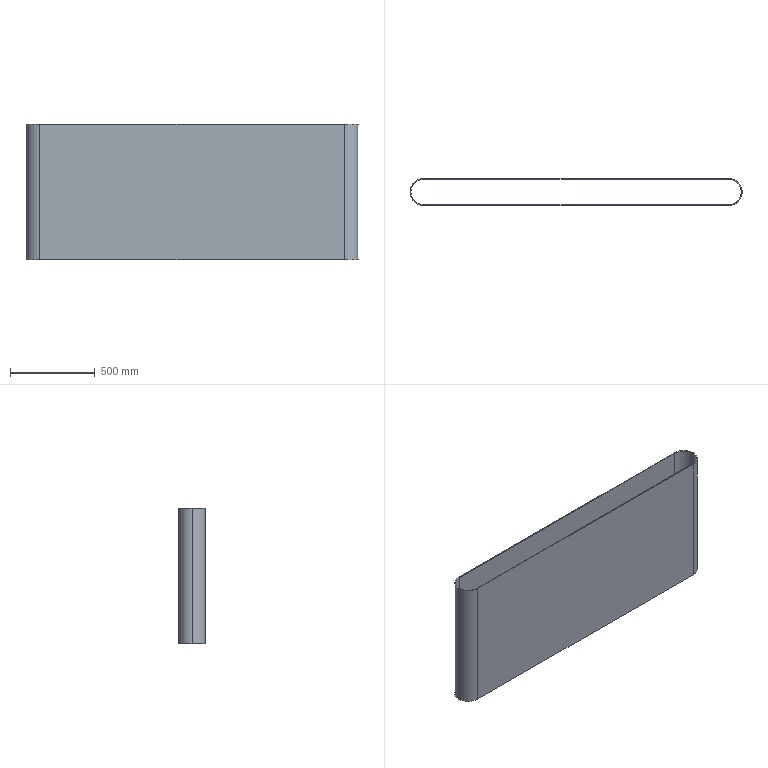Part | SolidWorks | features ExtruThin 1 | 1 solid | 12 faces | box 1960 x 160 x 800 mm | volume 16347787 mm3 | cylinder 6 | plane 6 | commonest cylinder face diameters 150 x3 160 x3
STEP:
#1=CARTESIAN_POINT('',(0.,75.,800.));
#2=VERTEX_POINT('',#1);
#3=CARTESIAN_POINT('',(-75.,0.,800.));
#4=VERTEX_POINT('',#3);
#5=CARTESIAN_POINT('',(0.,0.,800.));
#6=DIRECTION('',(0.,0.,1.));
#7=DIRECTION('',(1.,0.,0.));
#8=AXIS2_PLACEMENT_3D('',#5,#6,#7);
#9=CIRCLE('',#8,75.);
#10=EDGE_CURVE('',#2,#4,#9,.T.);
#11=ORIENTED_EDGE('',*,*,#10,.T.);
#12=CARTESIAN_POINT('',(-75.,0.,0.));
#13=VERTEX_POINT('',#12);
#14=CARTESIAN_POINT('',(-75.,0.,800.));
#15=DIRECTION('',(0.,0.,-1.));
#16=VECTOR('',#15,1000.);
#17=LINE('',#14,#16);
#18=EDGE_CURVE('',#4,#13,#17,.T.);
#19=ORIENTED_EDGE('',*,*,#18,.T.);
#20=CARTESIAN_POINT('',(0.,75.,0.));
#21=VERTEX_POINT('',#20);
#22=CARTESIAN_POINT('',(0.,0.,0.));
#23=DIRECTION('',(0.,0.,1.));
#24=DIRECTION('',(1.,0.,0.));
#25=AXIS2_PLACEMENT_3D('',#22,#23,#24);
#26=CIRCLE('',#25,75.);
#27=EDGE_CURVE('',#21,#13,#26,.T.);
#28=ORIENTED_EDGE('',*,*,#27,.F.);
#29=CARTESIAN_POINT('',(0.,75.,800.));
#30=DIRECTION('',(0.,0.,-1.));
#31=VECTOR('',#30,1000.);
#32=LINE('',#29,#31);
#33=EDGE_CURVE('',#2,#21,#32,.T.);
#34=ORIENTED_EDGE('',*,*,#33,.F.);
#35=EDGE_LOOP('',(#11,#19,#28,#34));
#36=FACE_OUTER_BOUND('',#35,.T.);
#37=CARTESIAN_POINT('',(0.,0.,800.));
#38=DIRECTION('',(0.,0.,-1.));
#39=DIRECTION('',(-1.,0.,0.));
#40=AXIS2_PLACEMENT_3D('',#37,#38,#39);
#41=CYLINDRICAL_SURFACE('',#40,75.);
#42=ADVANCED_FACE('',(#36),#41,.F.);
#43=CARTESIAN_POINT('',(-80.,0.,800.));
#44=VERTEX_POINT('',#43);
#45=CARTESIAN_POINT('',(0.,-80.,800.));
#46=VERTEX_POINT('',#45);
#47=CARTESIAN_POINT('',(0.,0.,800.));
#48=DIRECTION('',(0.,0.,1.));
#49=DIRECTION('',(1.,0.,0.));
#50=AXIS2_PLACEMENT_3D('',#47,#48,#49);
#51=CIRCLE('',#50,80.);
#52=EDGE_CURVE('',#44,#46,#51,.T.);
#53=ORIENTED_EDGE('',*,*,#52,.F.);
#54=CARTESIAN_POINT('',(-80.,0.,0.));
#55=VERTEX_POINT('',#54);
#56=CARTESIAN_POINT('',(-80.,0.,800.));
#57=DIRECTION('',(0.,0.,-1.));
#58=VECTOR('',#57,1000.);
#59=LINE('',#56,#58);
#60=EDGE_CURVE('',#44,#55,#59,.T.);
#61=ORIENTED_EDGE('',*,*,#60,.T.);
#62=CARTESIAN_POINT('',(0.,-80.,0.));
#63=VERTEX_POINT('',#62);
#64=CARTESIAN_POINT('',(0.,0.,0.));
#65=DIRECTION('',(0.,0.,1.));
#66=DIRECTION('',(1.,0.,0.));
#67=AXIS2_PLACEMENT_3D('',#64,#65,#66);
#68=CIRCLE('',#67,80.);
#69=EDGE_CURVE('',#55,#63,#68,.T.);
#70=ORIENTED_EDGE('',*,*,#69,.T.);
#71=CARTESIAN_POINT('',(0.,-80.,800.));
#72=DIRECTION('',(0.,0.,-1.));
#73=VECTOR('',#72,1000.);
#74=LINE('',#71,#73);
#75=EDGE_CURVE('',#46,#63,#74,.T.);
#76=ORIENTED_EDGE('',*,*,#75,.F.);
#77=EDGE_LOOP('',(#53,#61,#70,#76));
#78=FACE_OUTER_BOUND('',#77,.T.);
#79=CARTESIAN_POINT('',(0.,0.,800.));
#80=DIRECTION('',(0.,0.,-1.));
#81=DIRECTION('',(-1.,0.,0.));
#82=AXIS2_PLACEMENT_3D('',#79,#80,#81);
#83=CYLINDRICAL_SURFACE('',#82,80.);
#84=ADVANCED_FACE('',(#78),#83,.T.);
#85=CARTESIAN_POINT('',(0.,80.,800.));
#86=VERTEX_POINT('',#85);
#87=CARTESIAN_POINT('',(0.,0.,800.));
#88=DIRECTION('',(0.,0.,1.));
#89=DIRECTION('',(1.,0.,0.));
#90=AXIS2_PLACEMENT_3D('',#87,#88,#89);
#91=CIRCLE('',#90,80.);
#92=EDGE_CURVE('',#86,#44,#91,.T.);
#93=ORIENTED_EDGE('',*,*,#92,.T.);
#94=ORIENTED_EDGE('',*,*,#52,.T.);
#95=CARTESIAN_POINT('',(1800.,-80.,800.));
#96=VERTEX_POINT('',#95);
#97=CARTESIAN_POINT('',(0.,-80.,800.));
#98=DIRECTION('',(1.,0.,0.));
#99=VECTOR('',#98,1000.);
#100=LINE('',#97,#99);
#101=EDGE_CURVE('',#46,#96,#100,.T.);
#102=ORIENTED_EDGE('',*,*,#101,.T.);
#103=CARTESIAN_POINT('',(1800.,80.,800.));
#104=VERTEX_POINT('',#103);
#105=CARTESIAN_POINT('',(1800.,0.,800.));
#106=DIRECTION('',(0.,0.,1.));
#107=DIRECTION('',(1.,0.,0.));
#108=AXIS2_PLACEMENT_3D('',#105,#106,#107);
#109=CIRCLE('',#108,80.);
#110=EDGE_CURVE('',#96,#104,#109,.T.);
#111=ORIENTED_EDGE('',*,*,#110,.T.);
#112=CARTESIAN_POINT('',(0.,80.,800.));
#113=DIRECTION('',(1.,0.,0.));
#114=VECTOR('',#113,1000.);
#115=LINE('',#112,#114);
#116=EDGE_CURVE('',#86,#104,#115,.T.);
#117=ORIENTED_EDGE('',*,*,#116,.F.);
#118=EDGE_LOOP('',(#93,#94,#102,#111,#117));
#119=FACE_OUTER_BOUND('',#118,.T.);
#120=CARTESIAN_POINT('',(0.,-75.,800.));
#121=VERTEX_POINT('',#120);
#122=CARTESIAN_POINT('',(1800.,-75.,800.));
#123=VERTEX_POINT('',#122);
#124=CARTESIAN_POINT('',(0.,-75.,800.));
#125=DIRECTION('',(1.,0.,0.));
#126=VECTOR('',#125,1000.);
#127=LINE('',#124,#126);
#128=EDGE_CURVE('',#121,#123,#127,.T.);
#129=ORIENTED_EDGE('',*,*,#128,.F.);
#130=CARTESIAN_POINT('',(0.,0.,800.));
#131=DIRECTION('',(0.,0.,1.));
#132=DIRECTION('',(1.,0.,0.));
#133=AXIS2_PLACEMENT_3D('',#130,#131,#132);
#134=CIRCLE('',#133,75.);
#135=EDGE_CURVE('',#4,#121,#134,.T.);
#136=ORIENTED_EDGE('',*,*,#135,.F.);
#137=ORIENTED_EDGE('',*,*,#10,.F.);
#138=CARTESIAN_POINT('',(1800.,75.,800.));
#139=VERTEX_POINT('',#138);
#140=CARTESIAN_POINT('',(0.,75.,800.));
#141=DIRECTION('',(1.,0.,0.));
#142=VECTOR('',#141,1000.);
#143=LINE('',#140,#142);
#144=EDGE_CURVE('',#2,#139,#143,.T.);
#145=ORIENTED_EDGE('',*,*,#144,.T.);
#146=CARTESIAN_POINT('',(1800.,0.,800.));
#147=DIRECTION('',(0.,0.,1.));
#148=DIRECTION('',(1.,0.,0.));
#149=AXIS2_PLACEMENT_3D('',#146,#147,#148);
#150=CIRCLE('',#149,75.);
#151=EDGE_CURVE('',#123,#139,#150,.T.);
#152=ORIENTED_EDGE('',*,*,#151,.F.);
#153=EDGE_LOOP('',(#129,#136,#137,#145,#152));
#154=FACE_BOUND('',#153,.T.);
#155=CARTESIAN_POINT('',(0.,0.,800.));
#156=DIRECTION('',(0.,0.,1.));
#157=DIRECTION('',(1.,0.,0.));
#158=AXIS2_PLACEMENT_3D('',#155,#156,#157);
#159=PLANE('',#158);
#160=ADVANCED_FACE('',(#119,#154),#159,.T.);
#161=CARTESIAN_POINT('',(0.,80.,0.));
#162=VERTEX_POINT('',#161);
#163=CARTESIAN_POINT('',(0.,0.,0.));
#164=DIRECTION('',(0.,0.,1.));
#165=DIRECTION('',(1.,0.,0.));
#166=AXIS2_PLACEMENT_3D('',#163,#164,#165);
#167=CIRCLE('',#166,80.);
#168=EDGE_CURVE('',#162,#55,#167,.T.);
#169=ORIENTED_EDGE('',*,*,#168,.F.);
#170=CARTESIAN_POINT('',(1800.,80.,0.));
#171=VERTEX_POINT('',#170);
#172=CARTESIAN_POINT('',(0.,80.,0.));
#173=DIRECTION('',(1.,0.,0.));
#174=VECTOR('',#173,1000.);
#175=LINE('',#172,#174);
#176=EDGE_CURVE('',#162,#171,#175,.T.);
#177=ORIENTED_EDGE('',*,*,#176,.T.);
#178=CARTESIAN_POINT('',(1800.,-80.,0.));
#179=VERTEX_POINT('',#178);
#180=CARTESIAN_POINT('',(1800.,0.,0.));
#181=DIRECTION('',(0.,0.,1.));
#182=DIRECTION('',(1.,0.,0.));
#183=AXIS2_PLACEMENT_3D('',#180,#181,#182);
#184=CIRCLE('',#183,80.);
#185=EDGE_CURVE('',#179,#171,#184,.T.);
#186=ORIENTED_EDGE('',*,*,#185,.F.);
#187=CARTESIAN_POINT('',(0.,-80.,0.));
#188=DIRECTION('',(1.,0.,0.));
#189=VECTOR('',#188,1000.);
#190=LINE('',#187,#189);
#191=EDGE_CURVE('',#63,#179,#190,.T.);
#192=ORIENTED_EDGE('',*,*,#191,.F.);
#193=ORIENTED_EDGE('',*,*,#69,.F.);
#194=EDGE_LOOP('',(#169,#177,#186,#192,#193));
#195=FACE_OUTER_BOUND('',#194,.T.);
#196=ORIENTED_EDGE('',*,*,#27,.T.);
#197=CARTESIAN_POINT('',(0.,-75.,0.));
#198=VERTEX_POINT('',#197);
#199=CARTESIAN_POINT('',(0.,0.,0.));
#200=DIRECTION('',(0.,0.,1.));
#201=DIRECTION('',(1.,0.,0.));
#202=AXIS2_PLACEMENT_3D('',#199,#200,#201);
#203=CIRCLE('',#202,75.);
#204=EDGE_CURVE('',#13,#198,#203,.T.);
#205=ORIENTED_EDGE('',*,*,#204,.T.);
#206=CARTESIAN_POINT('',(1800.,-75.,0.));
#207=VERTEX_POINT('',#206);
#208=CARTESIAN_POINT('',(0.,-75.,0.));
#209=DIRECTION('',(1.,0.,0.));
#210=VECTOR('',#209,1000.);
#211=LINE('',#208,#210);
#212=EDGE_CURVE('',#198,#207,#211,.T.);
#213=ORIENTED_EDGE('',*,*,#212,.T.);
#214=CARTESIAN_POINT('',(1800.,75.,0.));
#215=VERTEX_POINT('',#214);
#216=CARTESIAN_POINT('',(1800.,0.,0.));
#217=DIRECTION('',(0.,0.,1.));
#218=DIRECTION('',(1.,0.,0.));
#219=AXIS2_PLACEMENT_3D('',#216,#217,#218);
#220=CIRCLE('',#219,75.);
#221=EDGE_CURVE('',#207,#215,#220,.T.);
#222=ORIENTED_EDGE('',*,*,#221,.T.);
#223=CARTESIAN_POINT('',(0.,75.,0.));
#224=DIRECTION('',(1.,0.,0.));
#225=VECTOR('',#224,1000.);
#226=LINE('',#223,#225);
#227=EDGE_CURVE('',#21,#215,#226,.T.);
#228=ORIENTED_EDGE('',*,*,#227,.F.);
#229=EDGE_LOOP('',(#196,#205,#213,#222,#228));
#230=FACE_BOUND('',#229,.T.);
#231=CARTESIAN_POINT('',(0.,0.,0.));
#232=DIRECTION('',(0.,0.,1.));
#233=DIRECTION('',(1.,0.,0.));
#234=AXIS2_PLACEMENT_3D('',#231,#232,#233);
#235=PLANE('',#234);
#236=ADVANCED_FACE('',(#195,#230),#235,.F.);
#237=ORIENTED_EDGE('',*,*,#60,.F.);
#238=ORIENTED_EDGE('',*,*,#92,.F.);
#239=CARTESIAN_POINT('',(0.,80.,800.));
#240=DIRECTION('',(0.,0.,-1.));
#241=VECTOR('',#240,1000.);
#242=LINE('',#239,#241);
#243=EDGE_CURVE('',#86,#162,#242,.T.);
#244=ORIENTED_EDGE('',*,*,#243,.T.);
#245=ORIENTED_EDGE('',*,*,#168,.T.);
#246=EDGE_LOOP('',(#237,#238,#244,#245));
#247=FACE_OUTER_BOUND('',#246,.T.);
#248=CARTESIAN_POINT('',(0.,0.,800.));
#249=DIRECTION('',(0.,0.,-1.));
#250=DIRECTION('',(-1.,0.,0.));
#251=AXIS2_PLACEMENT_3D('',#248,#249,#250);
#252=CYLINDRICAL_SURFACE('',#251,80.);
#253=ADVANCED_FACE('',(#247),#252,.T.);
#254=ORIENTED_EDGE('',*,*,#191,.T.);
#255=CARTESIAN_POINT('',(1800.,-80.,800.));
#256=DIRECTION('',(0.,0.,-1.));
#257=VECTOR('',#256,1000.);
#258=LINE('',#255,#257);
#259=EDGE_CURVE('',#96,#179,#258,.T.);
#260=ORIENTED_EDGE('',*,*,#259,.F.);
#261=ORIENTED_EDGE('',*,*,#101,.F.);
#262=ORIENTED_EDGE('',*,*,#75,.T.);
#263=EDGE_LOOP('',(#254,#260,#261,#262));
#264=FACE_OUTER_BOUND('',#263,.T.);
#265=CARTESIAN_POINT('',(0.,-80.,800.));
#266=DIRECTION('',(0.,1.,0.));
#267=DIRECTION('',(0.,0.,1.));
#268=AXIS2_PLACEMENT_3D('',#265,#266,#267);
#269=PLANE('',#268);
#270=ADVANCED_FACE('',(#264),#269,.F.);
#271=ORIENTED_EDGE('',*,*,#185,.T.);
#272=CARTESIAN_POINT('',(1800.,80.,800.));
#273=DIRECTION('',(0.,0.,-1.));
#274=VECTOR('',#273,1000.);
#275=LINE('',#272,#274);
#276=EDGE_CURVE('',#104,#171,#275,.T.);
#277=ORIENTED_EDGE('',*,*,#276,.F.);
#278=ORIENTED_EDGE('',*,*,#110,.F.);
#279=ORIENTED_EDGE('',*,*,#259,.T.);
#280=EDGE_LOOP('',(#271,#277,#278,#279));
#281=FACE_OUTER_BOUND('',#280,.T.);
#282=CARTESIAN_POINT('',(1800.,0.,800.));
#283=DIRECTION('',(0.,0.,-1.));
#284=DIRECTION('',(-1.,0.,0.));
#285=AXIS2_PLACEMENT_3D('',#282,#283,#284);
#286=CYLINDRICAL_SURFACE('',#285,80.);
#287=ADVANCED_FACE('',(#281),#286,.T.);
#288=ORIENTED_EDGE('',*,*,#176,.F.);
#289=ORIENTED_EDGE('',*,*,#243,.F.);
#290=ORIENTED_EDGE('',*,*,#116,.T.);
#291=ORIENTED_EDGE('',*,*,#276,.T.);
#292=EDGE_LOOP('',(#288,#289,#290,#291));
#293=FACE_OUTER_BOUND('',#292,.T.);
#294=CARTESIAN_POINT('',(0.,80.,800.));
#295=DIRECTION('',(0.,1.,0.));
#296=DIRECTION('',(0.,0.,1.));
#297=AXIS2_PLACEMENT_3D('',#294,#295,#296);
#298=PLANE('',#297);
#299=ADVANCED_FACE('',(#293),#298,.T.);
#300=ORIENTED_EDGE('',*,*,#18,.F.);
#301=ORIENTED_EDGE('',*,*,#135,.T.);
#302=CARTESIAN_POINT('',(0.,-75.,800.));
#303=DIRECTION('',(0.,0.,-1.));
#304=VECTOR('',#303,1000.);
#305=LINE('',#302,#304);
#306=EDGE_CURVE('',#121,#198,#305,.T.);
#307=ORIENTED_EDGE('',*,*,#306,.T.);
#308=ORIENTED_EDGE('',*,*,#204,.F.);
#309=EDGE_LOOP('',(#300,#301,#307,#308));
#310=FACE_OUTER_BOUND('',#309,.T.);
#311=CARTESIAN_POINT('',(0.,0.,800.));
#312=DIRECTION('',(0.,0.,-1.));
#313=DIRECTION('',(-1.,0.,0.));
#314=AXIS2_PLACEMENT_3D('',#311,#312,#313);
#315=CYLINDRICAL_SURFACE('',#314,75.);
#316=ADVANCED_FACE('',(#310),#315,.F.);
#317=ORIENTED_EDGE('',*,*,#212,.F.);
#318=ORIENTED_EDGE('',*,*,#306,.F.);
#319=ORIENTED_EDGE('',*,*,#128,.T.);
#320=CARTESIAN_POINT('',(1800.,-75.,800.));
#321=DIRECTION('',(0.,0.,-1.));
#322=VECTOR('',#321,1000.);
#323=LINE('',#320,#322);
#324=EDGE_CURVE('',#123,#207,#323,.T.);
#325=ORIENTED_EDGE('',*,*,#324,.T.);
#326=EDGE_LOOP('',(#317,#318,#319,#325));
#327=FACE_OUTER_BOUND('',#326,.T.);
#328=CARTESIAN_POINT('',(0.,-75.,800.));
#329=DIRECTION('',(0.,1.,0.));
#330=DIRECTION('',(0.,0.,1.));
#331=AXIS2_PLACEMENT_3D('',#328,#329,#330);
#332=PLANE('',#331);
#333=ADVANCED_FACE('',(#327),#332,.T.);
#334=ORIENTED_EDGE('',*,*,#221,.F.);
#335=ORIENTED_EDGE('',*,*,#324,.F.);
#336=ORIENTED_EDGE('',*,*,#151,.T.);
#337=CARTESIAN_POINT('',(1800.,75.,800.));
#338=DIRECTION('',(0.,0.,-1.));
#339=VECTOR('',#338,1000.);
#340=LINE('',#337,#339);
#341=EDGE_CURVE('',#139,#215,#340,.T.);
#342=ORIENTED_EDGE('',*,*,#341,.T.);
#343=EDGE_LOOP('',(#334,#335,#336,#342));
#344=FACE_OUTER_BOUND('',#343,.T.);
#345=CARTESIAN_POINT('',(1800.,0.,800.));
#346=DIRECTION('',(0.,0.,-1.));
#347=DIRECTION('',(-1.,0.,0.));
#348=AXIS2_PLACEMENT_3D('',#345,#346,#347);
#349=CYLINDRICAL_SURFACE('',#348,75.);
#350=ADVANCED_FACE('',(#344),#349,.F.);
#351=ORIENTED_EDGE('',*,*,#227,.T.);
#352=ORIENTED_EDGE('',*,*,#341,.F.);
#353=ORIENTED_EDGE('',*,*,#144,.F.);
#354=ORIENTED_EDGE('',*,*,#33,.T.);
#355=EDGE_LOOP('',(#351,#352,#353,#354));
#356=FACE_OUTER_BOUND('',#355,.T.);
#357=CARTESIAN_POINT('',(0.,75.,800.));
#358=DIRECTION('',(0.,1.,0.));
#359=DIRECTION('',(0.,0.,1.));
#360=AXIS2_PLACEMENT_3D('',#357,#358,#359);
#361=PLANE('',#360);
#362=ADVANCED_FACE('',(#356),#361,.F.);
#363=CLOSED_SHELL('',(#42,#84,#160,#236,#253,#270,#287,#299,#316,#333,#350,#362));
#364=MANIFOLD_SOLID_BREP('',#363);
#365=CARTESIAN_POINT('',(0.,0.,0.));
#366=DIRECTION('',(0.,0.,1.));
#367=DIRECTION('',(1.,0.,0.));
#368=AXIS2_PLACEMENT_3D('',#365,#366,#367);
#369=(LENGTH_UNIT()NAMED_UNIT(*)SI_UNIT(.MILLI.,.METRE.));
#370=UNCERTAINTY_MEASURE_WITH_UNIT(LENGTH_MEASURE(0.00001),#369,'','');
#371=(NAMED_UNIT(*)PLANE_ANGLE_UNIT()SI_UNIT($,.RADIAN.));
#372=(NAMED_UNIT(*)SI_UNIT($,.STERADIAN.)SOLID_ANGLE_UNIT());
#373=(GEOMETRIC_REPRESENTATION_CONTEXT(3)GLOBAL_UNCERTAINTY_ASSIGNED_CONTEXT((#370))GLOBAL_UNIT_ASSIGNED_CONTEXT((#369,#371,#372))REPRESENTATION_CONTEXT('',''));
#374=ADVANCED_BREP_SHAPE_REPRESENTATION('',(#364,#368),#373);